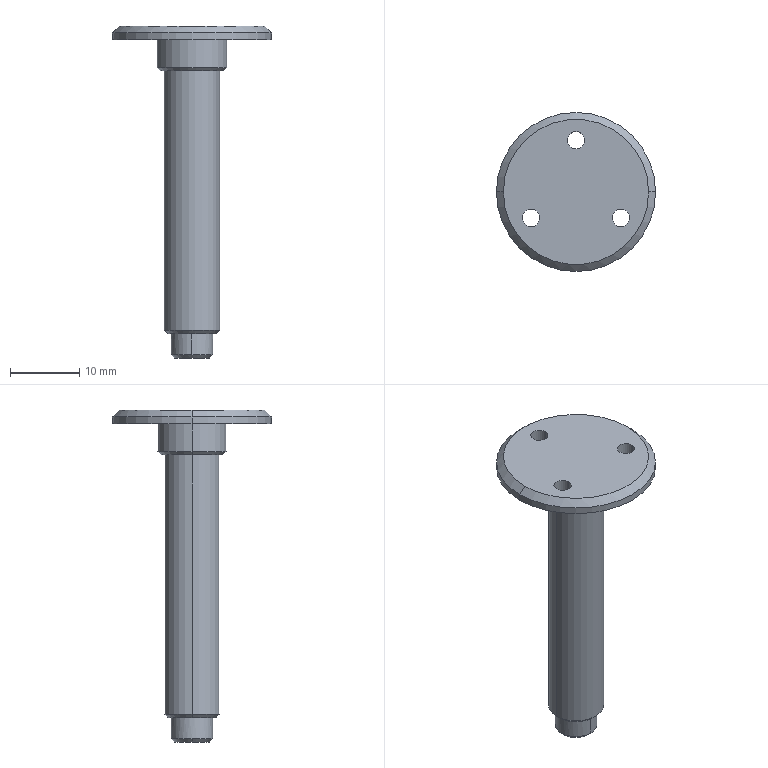Part | NX | features BREP 1 | 1 solid | 30 faces | box 23 x 23 x 48 mm | volume 3023 mm3 | cylinder 16 | cone 8 | plane 6 | commonest cylinder face diameters 2.5 x6 3.2 x2 6 x2 8 x2 10 x2 23 x2
STEP:
#1=CARTESIAN_POINT('',(100.41,208.217,0.));
#2=VERTEX_POINT('',#1);
#3=CARTESIAN_POINT('',(109.41,208.217,0.));
#4=VERTEX_POINT('',#3);
#5=CARTESIAN_POINT('',(104.91,208.217,0.));
#6=DIRECTION('',(0.,0.,-1.));
#7=DIRECTION('',(1.,0.,0.));
#8=AXIS2_PLACEMENT_3D('',#5,#6,#7);
#9=CIRCLE('',#8,4.5);
#10=EDGE_CURVE('',#2,#4,#9,.T.);
#11=ORIENTED_EDGE('',*,*,#10,.F.);
#12=CARTESIAN_POINT('',(99.91,208.217,0.5));
#13=VERTEX_POINT('',#12);
#14=CARTESIAN_POINT('',(99.91,208.217,0.5));
#15=DIRECTION('',(-0.7071,0.,0.7071));
#16=VECTOR('',#15,1000.);
#17=LINE('',#14,#16);
#18=EDGE_CURVE('',#2,#13,#17,.T.);
#19=ORIENTED_EDGE('',*,*,#18,.T.);
#20=CARTESIAN_POINT('',(109.91,208.217,0.5));
#21=VERTEX_POINT('',#20);
#22=CARTESIAN_POINT('',(104.91,208.217,0.5));
#23=DIRECTION('',(0.,0.,1.));
#24=DIRECTION('',(1.,0.,0.));
#25=AXIS2_PLACEMENT_3D('',#22,#23,#24);
#26=CIRCLE('',#25,5.);
#27=EDGE_CURVE('',#21,#13,#26,.T.);
#28=ORIENTED_EDGE('',*,*,#27,.F.);
#29=CARTESIAN_POINT('',(109.91,208.217,0.5));
#30=DIRECTION('',(0.7071,0.,0.7071));
#31=VECTOR('',#30,1000.);
#32=LINE('',#29,#31);
#33=EDGE_CURVE('',#4,#21,#32,.T.);
#34=ORIENTED_EDGE('',*,*,#33,.F.);
#35=EDGE_LOOP('',(#11,#19,#28,#34));
#36=FACE_BOUND('',#35,.T.);
#37=CARTESIAN_POINT('',(104.91,208.217,0.5));
#38=DIRECTION('',(0.,0.,1.));
#39=DIRECTION('',(-1.,0.,0.));
#40=AXIS2_PLACEMENT_3D('',#37,#38,#39);
#41=CONICAL_SURFACE('',#40,5.,0.7854);
#42=ADVANCED_FACE('',(#36),#41,.T.);
#43=CARTESIAN_POINT('',(102.41,208.217,-41.5));
#44=VERTEX_POINT('',#43);
#45=CARTESIAN_POINT('',(107.41,208.217,-41.5));
#46=VERTEX_POINT('',#45);
#47=CARTESIAN_POINT('',(104.91,208.217,-41.5));
#48=DIRECTION('',(0.,0.,-1.));
#49=DIRECTION('',(0.,1.,0.));
#50=AXIS2_PLACEMENT_3D('',#47,#48,#49);
#51=CIRCLE('',#50,2.5);
#52=EDGE_CURVE('',#44,#46,#51,.T.);
#53=ORIENTED_EDGE('',*,*,#52,.F.);
#54=CARTESIAN_POINT('',(101.91,208.217,-41.));
#55=VERTEX_POINT('',#54);
#56=CARTESIAN_POINT('',(102.41,208.217,-41.5));
#57=DIRECTION('',(-0.7071,0.,0.7071));
#58=VECTOR('',#57,1000.);
#59=LINE('',#56,#58);
#60=EDGE_CURVE('',#44,#55,#59,.T.);
#61=ORIENTED_EDGE('',*,*,#60,.T.);
#62=CARTESIAN_POINT('',(104.91,211.217,-41.));
#63=VERTEX_POINT('',#62);
#64=CARTESIAN_POINT('',(104.91,208.217,-41.));
#65=DIRECTION('',(0.,0.,1.));
#66=DIRECTION('',(-1.,0.,0.));
#67=AXIS2_PLACEMENT_3D('',#64,#65,#66);
#68=CIRCLE('',#67,3.);
#69=EDGE_CURVE('',#63,#55,#68,.T.);
#70=ORIENTED_EDGE('',*,*,#69,.F.);
#71=CARTESIAN_POINT('',(107.91,208.217,-41.));
#72=VERTEX_POINT('',#71);
#73=CARTESIAN_POINT('',(104.91,208.217,-41.));
#74=DIRECTION('',(0.,0.,1.));
#75=DIRECTION('',(-1.,0.,0.));
#76=AXIS2_PLACEMENT_3D('',#73,#74,#75);
#77=CIRCLE('',#76,3.);
#78=EDGE_CURVE('',#72,#63,#77,.T.);
#79=ORIENTED_EDGE('',*,*,#78,.F.);
#80=CARTESIAN_POINT('',(107.41,208.217,-41.5));
#81=DIRECTION('',(0.7071,0.,0.7071));
#82=VECTOR('',#81,1000.);
#83=LINE('',#80,#82);
#84=EDGE_CURVE('',#46,#72,#83,.T.);
#85=ORIENTED_EDGE('',*,*,#84,.F.);
#86=EDGE_LOOP('',(#53,#61,#70,#79,#85));
#87=FACE_BOUND('',#86,.T.);
#88=CARTESIAN_POINT('',(104.91,208.217,-41.5));
#89=DIRECTION('',(0.,0.,1.));
#90=DIRECTION('',(-1.,0.,0.));
#91=AXIS2_PLACEMENT_3D('',#88,#89,#90);
#92=CONICAL_SURFACE('',#91,2.5,0.7854);
#93=ADVANCED_FACE('',(#87),#92,.T.);
#94=CARTESIAN_POINT('',(101.41,208.217,-38.));
#95=VERTEX_POINT('',#94);
#96=CARTESIAN_POINT('',(108.41,208.217,-38.));
#97=VERTEX_POINT('',#96);
#98=CARTESIAN_POINT('',(104.91,208.217,-38.));
#99=DIRECTION('',(0.,0.,-1.));
#100=DIRECTION('',(0.,1.,0.));
#101=AXIS2_PLACEMENT_3D('',#98,#99,#100);
#102=CIRCLE('',#101,3.5);
#103=EDGE_CURVE('',#95,#97,#102,.T.);
#104=ORIENTED_EDGE('',*,*,#103,.F.);
#105=CARTESIAN_POINT('',(100.91,208.217,-37.5));
#106=VERTEX_POINT('',#105);
#107=CARTESIAN_POINT('',(101.41,208.217,-38.));
#108=DIRECTION('',(-0.7071,0.,0.7071));
#109=VECTOR('',#108,1000.);
#110=LINE('',#107,#109);
#111=EDGE_CURVE('',#95,#106,#110,.T.);
#112=ORIENTED_EDGE('',*,*,#111,.T.);
#113=CARTESIAN_POINT('',(108.91,208.217,-37.5));
#114=VERTEX_POINT('',#113);
#115=CARTESIAN_POINT('',(104.91,208.217,-37.5));
#116=DIRECTION('',(0.,0.,1.));
#117=DIRECTION('',(-1.,0.,0.));
#118=AXIS2_PLACEMENT_3D('',#115,#116,#117);
#119=CIRCLE('',#118,4.);
#120=EDGE_CURVE('',#114,#106,#119,.T.);
#121=ORIENTED_EDGE('',*,*,#120,.F.);
#122=CARTESIAN_POINT('',(108.41,208.217,-38.));
#123=DIRECTION('',(0.7071,0.,0.7071));
#124=VECTOR('',#123,1000.);
#125=LINE('',#122,#124);
#126=EDGE_CURVE('',#97,#114,#125,.T.);
#127=ORIENTED_EDGE('',*,*,#126,.F.);
#128=EDGE_LOOP('',(#104,#112,#121,#127));
#129=FACE_BOUND('',#128,.T.);
#130=CARTESIAN_POINT('',(104.91,208.217,-38.));
#131=DIRECTION('',(0.,0.,1.));
#132=DIRECTION('',(-1.,0.,0.));
#133=AXIS2_PLACEMENT_3D('',#130,#131,#132);
#134=CONICAL_SURFACE('',#133,3.5,0.7854);
#135=ADVANCED_FACE('',(#129),#134,.T.);
#136=CARTESIAN_POINT('',(104.91,206.617,-29.5));
#137=VERTEX_POINT('',#136);
#138=CARTESIAN_POINT('',(104.91,209.817,-29.5));
#139=VERTEX_POINT('',#138);
#140=CARTESIAN_POINT('',(104.91,208.217,-29.5));
#141=DIRECTION('',(0.,0.,-1.));
#142=DIRECTION('',(0.,1.,0.));
#143=AXIS2_PLACEMENT_3D('',#140,#141,#142);
#144=CIRCLE('',#143,1.6);
#145=EDGE_CURVE('',#137,#139,#144,.T.);
#146=ORIENTED_EDGE('',*,*,#145,.F.);
#147=CARTESIAN_POINT('',(104.91,206.617,-41.5));
#148=VERTEX_POINT('',#147);
#149=CARTESIAN_POINT('',(104.91,206.617,-29.5));
#150=DIRECTION('',(0.,0.,-1.));
#151=VECTOR('',#150,1000.);
#152=LINE('',#149,#151);
#153=EDGE_CURVE('',#137,#148,#152,.T.);
#154=ORIENTED_EDGE('',*,*,#153,.T.);
#155=CARTESIAN_POINT('',(104.91,209.817,-41.5));
#156=VERTEX_POINT('',#155);
#157=CARTESIAN_POINT('',(104.91,208.217,-41.5));
#158=DIRECTION('',(0.,0.,-1.));
#159=DIRECTION('',(0.,1.,0.));
#160=AXIS2_PLACEMENT_3D('',#157,#158,#159);
#161=CIRCLE('',#160,1.6);
#162=EDGE_CURVE('',#148,#156,#161,.T.);
#163=ORIENTED_EDGE('',*,*,#162,.T.);
#164=CARTESIAN_POINT('',(104.91,209.817,-29.5));
#165=DIRECTION('',(0.,0.,-1.));
#166=VECTOR('',#165,1000.);
#167=LINE('',#164,#166);
#168=EDGE_CURVE('',#139,#156,#167,.T.);
#169=ORIENTED_EDGE('',*,*,#168,.F.);
#170=EDGE_LOOP('',(#146,#154,#163,#169));
#171=FACE_BOUND('',#170,.T.);
#172=CARTESIAN_POINT('',(104.91,208.217,-29.5));
#173=DIRECTION('',(0.,0.,-1.));
#174=DIRECTION('',(0.,-1.,0.));
#175=AXIS2_PLACEMENT_3D('',#172,#173,#174);
#176=CYLINDRICAL_SURFACE('',#175,1.6);
#177=ADVANCED_FACE('',(#171),#176,.F.);
#178=CARTESIAN_POINT('',(104.91,211.217,-38.));
#179=VERTEX_POINT('',#178);
#180=CARTESIAN_POINT('',(104.91,205.217,-38.));
#181=VERTEX_POINT('',#180);
#182=CARTESIAN_POINT('',(104.91,208.217,-38.));
#183=DIRECTION('',(0.,0.,-1.));
#184=DIRECTION('',(0.5022,0.8648,0.));
#185=AXIS2_PLACEMENT_3D('',#182,#183,#184);
#186=CIRCLE('',#185,3.);
#187=EDGE_CURVE('',#179,#181,#186,.T.);
#188=ORIENTED_EDGE('',*,*,#187,.T.);
#189=CARTESIAN_POINT('',(104.91,205.217,-41.));
#190=VERTEX_POINT('',#189);
#191=CARTESIAN_POINT('',(104.91,205.217,-22.075));
#192=DIRECTION('',(0.,0.,-1.));
#193=VECTOR('',#192,1000.);
#194=LINE('',#191,#193);
#195=EDGE_CURVE('',#181,#190,#194,.T.);
#196=ORIENTED_EDGE('',*,*,#195,.T.);
#197=CARTESIAN_POINT('',(104.91,208.217,-41.));
#198=DIRECTION('',(0.,0.,1.));
#199=DIRECTION('',(-1.,0.,0.));
#200=AXIS2_PLACEMENT_3D('',#197,#198,#199);
#201=CIRCLE('',#200,3.);
#202=EDGE_CURVE('',#190,#72,#201,.T.);
#203=ORIENTED_EDGE('',*,*,#202,.T.);
#204=ORIENTED_EDGE('',*,*,#78,.T.);
#205=CARTESIAN_POINT('',(104.91,211.217,-22.075));
#206=DIRECTION('',(0.,0.,-1.));
#207=VECTOR('',#206,1000.);
#208=LINE('',#205,#207);
#209=EDGE_CURVE('',#179,#63,#208,.T.);
#210=ORIENTED_EDGE('',*,*,#209,.F.);
#211=EDGE_LOOP('',(#188,#196,#203,#204,#210));
#212=FACE_BOUND('',#211,.T.);
#213=CARTESIAN_POINT('',(104.91,208.217,-22.075));
#214=DIRECTION('',(0.,0.,-1.));
#215=DIRECTION('',(0.,-1.,0.));
#216=AXIS2_PLACEMENT_3D('',#213,#214,#215);
#217=CYLINDRICAL_SURFACE('',#216,3.);
#218=ADVANCED_FACE('',(#212),#217,.T.);
#219=CARTESIAN_POINT('',(115.41,208.217,6.5));
#220=VERTEX_POINT('',#219);
#221=CARTESIAN_POINT('',(94.41,208.217,6.5));
#222=VERTEX_POINT('',#221);
#223=CARTESIAN_POINT('',(104.91,208.217,6.5));
#224=DIRECTION('',(0.,0.,1.));
#225=DIRECTION('',(1.,0.,0.));
#226=AXIS2_PLACEMENT_3D('',#223,#224,#225);
#227=CIRCLE('',#226,10.5);
#228=EDGE_CURVE('',#220,#222,#227,.T.);
#229=ORIENTED_EDGE('',*,*,#228,.F.);
#230=CARTESIAN_POINT('',(116.41,208.217,5.5));
#231=VERTEX_POINT('',#230);
#232=CARTESIAN_POINT('',(115.41,208.217,6.5));
#233=DIRECTION('',(0.7071,0.,-0.7071));
#234=VECTOR('',#233,1000.);
#235=LINE('',#232,#234);
#236=EDGE_CURVE('',#231,#220,#235,.F.);
#237=ORIENTED_EDGE('',*,*,#236,.F.);
#238=CARTESIAN_POINT('',(93.41,208.217,5.5));
#239=VERTEX_POINT('',#238);
#240=CARTESIAN_POINT('',(104.91,208.217,5.5));
#241=DIRECTION('',(0.,0.,-1.));
#242=DIRECTION('',(1.,0.,0.));
#243=AXIS2_PLACEMENT_3D('',#240,#241,#242);
#244=CIRCLE('',#243,11.5);
#245=EDGE_CURVE('',#239,#231,#244,.T.);
#246=ORIENTED_EDGE('',*,*,#245,.F.);
#247=CARTESIAN_POINT('',(94.41,208.217,6.5));
#248=DIRECTION('',(-0.7071,0.,-0.7071));
#249=VECTOR('',#248,1000.);
#250=LINE('',#247,#249);
#251=EDGE_CURVE('',#239,#222,#250,.F.);
#252=ORIENTED_EDGE('',*,*,#251,.T.);
#253=EDGE_LOOP('',(#229,#237,#246,#252));
#254=FACE_BOUND('',#253,.T.);
#255=CARTESIAN_POINT('',(104.91,208.217,6.5));
#256=DIRECTION('',(0.,0.,-1.));
#257=DIRECTION('',(1.,0.,0.));
#258=AXIS2_PLACEMENT_3D('',#255,#256,#257);
#259=CONICAL_SURFACE('',#258,10.5,0.7854);
#260=ADVANCED_FACE('',(#254),#259,.T.);
#261=CARTESIAN_POINT('',(97.165,204.467,6.5));
#262=VERTEX_POINT('',#261);
#263=CARTESIAN_POINT('',(99.665,204.467,6.5));
#264=VERTEX_POINT('',#263);
#265=CARTESIAN_POINT('',(98.415,204.467,6.5));
#266=DIRECTION('',(0.,0.,1.));
#267=DIRECTION('',(1.,0.,0.));
#268=AXIS2_PLACEMENT_3D('',#265,#266,#267);
#269=CIRCLE('',#268,1.25);
#270=EDGE_CURVE('',#262,#264,#269,.T.);
#271=ORIENTED_EDGE('',*,*,#270,.T.);
#272=CARTESIAN_POINT('',(99.665,204.467,4.5));
#273=VERTEX_POINT('',#272);
#274=CARTESIAN_POINT('',(99.665,204.467,6.5));
#275=DIRECTION('',(0.,0.,-1.));
#276=VECTOR('',#275,1000.);
#277=LINE('',#274,#276);
#278=EDGE_CURVE('',#273,#264,#277,.F.);
#279=ORIENTED_EDGE('',*,*,#278,.F.);
#280=CARTESIAN_POINT('',(97.165,204.467,4.5));
#281=VERTEX_POINT('',#280);
#282=CARTESIAN_POINT('',(98.415,204.467,4.5));
#283=DIRECTION('',(0.,0.,1.));
#284=DIRECTION('',(1.,0.,0.));
#285=AXIS2_PLACEMENT_3D('',#282,#283,#284);
#286=CIRCLE('',#285,1.25);
#287=EDGE_CURVE('',#281,#273,#286,.T.);
#288=ORIENTED_EDGE('',*,*,#287,.F.);
#289=CARTESIAN_POINT('',(97.165,204.467,6.5));
#290=DIRECTION('',(0.,0.,-1.));
#291=VECTOR('',#290,1000.);
#292=LINE('',#289,#291);
#293=EDGE_CURVE('',#281,#262,#292,.F.);
#294=ORIENTED_EDGE('',*,*,#293,.T.);
#295=EDGE_LOOP('',(#271,#279,#288,#294));
#296=FACE_BOUND('',#295,.T.);
#297=CARTESIAN_POINT('',(98.415,204.467,6.5));
#298=DIRECTION('',(0.,0.,-1.));
#299=DIRECTION('',(1.,0.,0.));
#300=AXIS2_PLACEMENT_3D('',#297,#298,#299);
#301=CYLINDRICAL_SURFACE('',#300,1.25);
#302=ADVANCED_FACE('',(#296),#301,.F.);
#303=CARTESIAN_POINT('',(110.155,204.467,6.5));
#304=VERTEX_POINT('',#303);
#305=CARTESIAN_POINT('',(112.655,204.467,6.5));
#306=VERTEX_POINT('',#305);
#307=CARTESIAN_POINT('',(111.405,204.467,6.5));
#308=DIRECTION('',(0.,0.,1.));
#309=DIRECTION('',(1.,0.,0.));
#310=AXIS2_PLACEMENT_3D('',#307,#308,#309);
#311=CIRCLE('',#310,1.25);
#312=EDGE_CURVE('',#304,#306,#311,.T.);
#313=ORIENTED_EDGE('',*,*,#312,.T.);
#314=CARTESIAN_POINT('',(112.655,204.467,4.5));
#315=VERTEX_POINT('',#314);
#316=CARTESIAN_POINT('',(112.655,204.467,6.5));
#317=DIRECTION('',(0.,0.,-1.));
#318=VECTOR('',#317,1000.);
#319=LINE('',#316,#318);
#320=EDGE_CURVE('',#315,#306,#319,.F.);
#321=ORIENTED_EDGE('',*,*,#320,.F.);
#322=CARTESIAN_POINT('',(110.155,204.467,4.5));
#323=VERTEX_POINT('',#322);
#324=CARTESIAN_POINT('',(111.405,204.467,4.5));
#325=DIRECTION('',(0.,0.,1.));
#326=DIRECTION('',(1.,0.,0.));
#327=AXIS2_PLACEMENT_3D('',#324,#325,#326);
#328=CIRCLE('',#327,1.25);
#329=EDGE_CURVE('',#323,#315,#328,.T.);
#330=ORIENTED_EDGE('',*,*,#329,.F.);
#331=CARTESIAN_POINT('',(110.155,204.467,6.5));
#332=DIRECTION('',(0.,0.,-1.));
#333=VECTOR('',#332,1000.);
#334=LINE('',#331,#333);
#335=EDGE_CURVE('',#323,#304,#334,.F.);
#336=ORIENTED_EDGE('',*,*,#335,.T.);
#337=EDGE_LOOP('',(#313,#321,#330,#336));
#338=FACE_BOUND('',#337,.T.);
#339=CARTESIAN_POINT('',(111.405,204.467,6.5));
#340=DIRECTION('',(0.,0.,-1.));
#341=DIRECTION('',(1.,0.,0.));
#342=AXIS2_PLACEMENT_3D('',#339,#340,#341);
#343=CYLINDRICAL_SURFACE('',#342,1.25);
#344=ADVANCED_FACE('',(#338),#343,.F.);
#345=CARTESIAN_POINT('',(103.66,215.717,6.5));
#346=VERTEX_POINT('',#345);
#347=CARTESIAN_POINT('',(106.16,215.717,6.5));
#348=VERTEX_POINT('',#347);
#349=CARTESIAN_POINT('',(104.91,215.717,6.5));
#350=DIRECTION('',(0.,0.,1.));
#351=DIRECTION('',(1.,0.,0.));
#352=AXIS2_PLACEMENT_3D('',#349,#350,#351);
#353=CIRCLE('',#352,1.25);
#354=EDGE_CURVE('',#346,#348,#353,.T.);
#355=ORIENTED_EDGE('',*,*,#354,.T.);
#356=CARTESIAN_POINT('',(106.16,215.717,4.5));
#357=VERTEX_POINT('',#356);
#358=CARTESIAN_POINT('',(106.16,215.717,6.5));
#359=DIRECTION('',(0.,0.,-1.));
#360=VECTOR('',#359,1000.);
#361=LINE('',#358,#360);
#362=EDGE_CURVE('',#357,#348,#361,.F.);
#363=ORIENTED_EDGE('',*,*,#362,.F.);
#364=CARTESIAN_POINT('',(103.66,215.717,4.5));
#365=VERTEX_POINT('',#364);
#366=CARTESIAN_POINT('',(104.91,215.717,4.5));
#367=DIRECTION('',(0.,0.,1.));
#368=DIRECTION('',(1.,0.,0.));
#369=AXIS2_PLACEMENT_3D('',#366,#367,#368);
#370=CIRCLE('',#369,1.25);
#371=EDGE_CURVE('',#365,#357,#370,.T.);
#372=ORIENTED_EDGE('',*,*,#371,.F.);
#373=CARTESIAN_POINT('',(103.66,215.717,6.5));
#374=DIRECTION('',(0.,0.,-1.));
#375=VECTOR('',#374,1000.);
#376=LINE('',#373,#375);
#377=EDGE_CURVE('',#365,#346,#376,.F.);
#378=ORIENTED_EDGE('',*,*,#377,.T.);
#379=EDGE_LOOP('',(#355,#363,#372,#378));
#380=FACE_BOUND('',#379,.T.);
#381=CARTESIAN_POINT('',(104.91,215.717,6.5));
#382=DIRECTION('',(0.,0.,-1.));
#383=DIRECTION('',(1.,0.,0.));
#384=AXIS2_PLACEMENT_3D('',#381,#382,#383);
#385=CYLINDRICAL_SURFACE('',#384,1.25);
#386=ADVANCED_FACE('',(#380),#385,.F.);
#387=ORIENTED_EDGE('',*,*,#245,.T.);
#388=CARTESIAN_POINT('',(116.41,208.217,4.5));
#389=VERTEX_POINT('',#388);
#390=CARTESIAN_POINT('',(116.41,208.217,6.5));
#391=DIRECTION('',(0.,0.,-1.));
#392=VECTOR('',#391,1000.);
#393=LINE('',#390,#392);
#394=EDGE_CURVE('',#389,#231,#393,.F.);
#395=ORIENTED_EDGE('',*,*,#394,.F.);
#396=CARTESIAN_POINT('',(93.41,208.217,4.5));
#397=VERTEX_POINT('',#396);
#398=CARTESIAN_POINT('',(104.91,208.217,4.5));
#399=DIRECTION('',(0.,0.,1.));
#400=DIRECTION('',(1.,0.,0.));
#401=AXIS2_PLACEMENT_3D('',#398,#399,#400);
#402=CIRCLE('',#401,11.5);
#403=EDGE_CURVE('',#389,#397,#402,.T.);
#404=ORIENTED_EDGE('',*,*,#403,.T.);
#405=CARTESIAN_POINT('',(93.41,208.217,6.5));
#406=DIRECTION('',(0.,0.,-1.));
#407=VECTOR('',#406,1000.);
#408=LINE('',#405,#407);
#409=EDGE_CURVE('',#397,#239,#408,.F.);
#410=ORIENTED_EDGE('',*,*,#409,.T.);
#411=EDGE_LOOP('',(#387,#395,#404,#410));
#412=FACE_BOUND('',#411,.T.);
#413=CARTESIAN_POINT('',(104.91,208.217,6.5));
#414=DIRECTION('',(0.,0.,-1.));
#415=DIRECTION('',(1.,0.,0.));
#416=AXIS2_PLACEMENT_3D('',#413,#414,#415);
#417=CYLINDRICAL_SURFACE('',#416,11.5);
#418=ADVANCED_FACE('',(#412),#417,.T.);
#419=CARTESIAN_POINT('',(99.91,208.217,4.5));
#420=VERTEX_POINT('',#419);
#421=CARTESIAN_POINT('',(109.91,208.217,4.5));
#422=VERTEX_POINT('',#421);
#423=CARTESIAN_POINT('',(104.91,208.217,4.5));
#424=DIRECTION('',(0.,0.,-1.));
#425=DIRECTION('',(0.,1.,0.));
#426=AXIS2_PLACEMENT_3D('',#423,#424,#425);
#427=CIRCLE('',#426,5.);
#428=EDGE_CURVE('',#420,#422,#427,.T.);
#429=ORIENTED_EDGE('',*,*,#428,.T.);
#430=CARTESIAN_POINT('',(109.91,208.217,18.642));
#431=DIRECTION('',(0.,0.,-1.));
#432=VECTOR('',#431,1000.);
#433=LINE('',#430,#432);
#434=EDGE_CURVE('',#21,#422,#433,.F.);
#435=ORIENTED_EDGE('',*,*,#434,.F.);
#436=ORIENTED_EDGE('',*,*,#27,.T.);
#437=CARTESIAN_POINT('',(99.91,208.217,18.642));
#438=DIRECTION('',(0.,0.,-1.));
#439=VECTOR('',#438,1000.);
#440=LINE('',#437,#439);
#441=EDGE_CURVE('',#13,#420,#440,.F.);
#442=ORIENTED_EDGE('',*,*,#441,.T.);
#443=EDGE_LOOP('',(#429,#435,#436,#442));
#444=FACE_BOUND('',#443,.T.);
#445=CARTESIAN_POINT('',(104.91,208.217,18.642));
#446=DIRECTION('',(0.,0.,-1.));
#447=DIRECTION('',(1.,0.,0.));
#448=AXIS2_PLACEMENT_3D('',#445,#446,#447);
#449=CYLINDRICAL_SURFACE('',#448,5.);
#450=ADVANCED_FACE('',(#444),#449,.T.);
#451=ORIENTED_EDGE('',*,*,#120,.T.);
#452=CARTESIAN_POINT('',(100.91,208.217,0.));
#453=VERTEX_POINT('',#452);
#454=CARTESIAN_POINT('',(100.91,208.217,-52.814));
#455=DIRECTION('',(0.,0.,1.));
#456=VECTOR('',#455,1000.);
#457=LINE('',#454,#456);
#458=EDGE_CURVE('',#106,#453,#457,.T.);
#459=ORIENTED_EDGE('',*,*,#458,.T.);
#460=CARTESIAN_POINT('',(108.91,208.217,0.));
#461=VERTEX_POINT('',#460);
#462=CARTESIAN_POINT('',(104.91,208.217,0.));
#463=DIRECTION('',(0.,0.,-1.));
#464=DIRECTION('',(-1.,0.,0.));
#465=AXIS2_PLACEMENT_3D('',#462,#463,#464);
#466=CIRCLE('',#465,4.);
#467=EDGE_CURVE('',#453,#461,#466,.T.);
#468=ORIENTED_EDGE('',*,*,#467,.T.);
#469=CARTESIAN_POINT('',(108.91,208.217,-52.814));
#470=DIRECTION('',(0.,0.,1.));
#471=VECTOR('',#470,1000.);
#472=LINE('',#469,#471);
#473=EDGE_CURVE('',#114,#461,#472,.T.);
#474=ORIENTED_EDGE('',*,*,#473,.F.);
#475=EDGE_LOOP('',(#451,#459,#468,#474));
#476=FACE_BOUND('',#475,.T.);
#477=CARTESIAN_POINT('',(104.91,208.217,-52.814));
#478=DIRECTION('',(0.,0.,1.));
#479=DIRECTION('',(-1.,0.,0.));
#480=AXIS2_PLACEMENT_3D('',#477,#478,#479);
#481=CYLINDRICAL_SURFACE('',#480,4.);
#482=ADVANCED_FACE('',(#476),#481,.T.);
#483=ORIENTED_EDGE('',*,*,#458,.F.);
#484=CARTESIAN_POINT('',(104.91,208.217,-37.5));
#485=DIRECTION('',(0.,0.,1.));
#486=DIRECTION('',(-1.,0.,0.));
#487=AXIS2_PLACEMENT_3D('',#484,#485,#486);
#488=CIRCLE('',#487,4.);
#489=EDGE_CURVE('',#106,#114,#488,.T.);
#490=ORIENTED_EDGE('',*,*,#489,.T.);
#491=ORIENTED_EDGE('',*,*,#473,.T.);
#492=CARTESIAN_POINT('',(104.91,208.217,0.));
#493=DIRECTION('',(0.,0.,-1.));
#494=DIRECTION('',(-1.,0.,0.));
#495=AXIS2_PLACEMENT_3D('',#492,#493,#494);
#496=CIRCLE('',#495,4.);
#497=EDGE_CURVE('',#461,#453,#496,.T.);
#498=ORIENTED_EDGE('',*,*,#497,.T.);
#499=EDGE_LOOP('',(#483,#490,#491,#498));
#500=FACE_BOUND('',#499,.T.);
#501=CARTESIAN_POINT('',(104.91,208.217,-52.814));
#502=DIRECTION('',(0.,0.,1.));
#503=DIRECTION('',(-1.,0.,0.));
#504=AXIS2_PLACEMENT_3D('',#501,#502,#503);
#505=CYLINDRICAL_SURFACE('',#504,4.);
#506=ADVANCED_FACE('',(#500),#505,.T.);
#507=CARTESIAN_POINT('',(104.91,208.217,0.));
#508=DIRECTION('',(0.,0.,-1.));
#509=DIRECTION('',(1.,0.,0.));
#510=AXIS2_PLACEMENT_3D('',#507,#508,#509);
#511=CIRCLE('',#510,4.5);
#512=EDGE_CURVE('',#4,#2,#511,.T.);
#513=ORIENTED_EDGE('',*,*,#512,.T.);
#514=ORIENTED_EDGE('',*,*,#10,.T.);
#515=EDGE_LOOP('',(#513,#514));
#516=FACE_BOUND('',#515,.T.);
#517=ORIENTED_EDGE('',*,*,#497,.F.);
#518=ORIENTED_EDGE('',*,*,#467,.F.);
#519=EDGE_LOOP('',(#517,#518));
#520=FACE_BOUND('',#519,.T.);
#521=CARTESIAN_POINT('',(104.91,208.217,0.));
#522=DIRECTION('',(0.,0.,1.));
#523=DIRECTION('',(-1.,0.,0.));
#524=AXIS2_PLACEMENT_3D('',#521,#522,#523);
#525=PLANE('',#524);
#526=ADVANCED_FACE('',(#516,#520),#525,.F.);
#527=ORIENTED_EDGE('',*,*,#434,.T.);
#528=CARTESIAN_POINT('',(104.91,208.217,4.5));
#529=DIRECTION('',(0.,0.,-1.));
#530=DIRECTION('',(0.,1.,0.));
#531=AXIS2_PLACEMENT_3D('',#528,#529,#530);
#532=CIRCLE('',#531,5.);
#533=EDGE_CURVE('',#422,#420,#532,.T.);
#534=ORIENTED_EDGE('',*,*,#533,.T.);
#535=ORIENTED_EDGE('',*,*,#441,.F.);
#536=CARTESIAN_POINT('',(104.91,208.217,0.5));
#537=DIRECTION('',(0.,0.,1.));
#538=DIRECTION('',(1.,0.,0.));
#539=AXIS2_PLACEMENT_3D('',#536,#537,#538);
#540=CIRCLE('',#539,5.);
#541=EDGE_CURVE('',#13,#21,#540,.T.);
#542=ORIENTED_EDGE('',*,*,#541,.T.);
#543=EDGE_LOOP('',(#527,#534,#535,#542));
#544=FACE_BOUND('',#543,.T.);
#545=CARTESIAN_POINT('',(104.91,208.217,18.642));
#546=DIRECTION('',(0.,0.,-1.));
#547=DIRECTION('',(1.,0.,0.));
#548=AXIS2_PLACEMENT_3D('',#545,#546,#547);
#549=CYLINDRICAL_SURFACE('',#548,5.);
#550=ADVANCED_FACE('',(#544),#549,.T.);
#551=CARTESIAN_POINT('',(104.91,208.217,6.5));
#552=DIRECTION('',(0.,0.,1.));
#553=DIRECTION('',(1.,0.,0.));
#554=AXIS2_PLACEMENT_3D('',#551,#552,#553);
#555=CIRCLE('',#554,10.5);
#556=EDGE_CURVE('',#222,#220,#555,.T.);
#557=ORIENTED_EDGE('',*,*,#556,.T.);
#558=ORIENTED_EDGE('',*,*,#228,.T.);
#559=EDGE_LOOP('',(#557,#558));
#560=FACE_BOUND('',#559,.T.);
#561=ORIENTED_EDGE('',*,*,#312,.F.);
#562=CARTESIAN_POINT('',(111.405,204.467,6.5));
#563=DIRECTION('',(0.,0.,1.));
#564=DIRECTION('',(1.,0.,0.));
#565=AXIS2_PLACEMENT_3D('',#562,#563,#564);
#566=CIRCLE('',#565,1.25);
#567=EDGE_CURVE('',#306,#304,#566,.T.);
#568=ORIENTED_EDGE('',*,*,#567,.F.);
#569=EDGE_LOOP('',(#561,#568));
#570=FACE_BOUND('',#569,.T.);
#571=ORIENTED_EDGE('',*,*,#354,.F.);
#572=CARTESIAN_POINT('',(104.91,215.717,6.5));
#573=DIRECTION('',(0.,0.,1.));
#574=DIRECTION('',(1.,0.,0.));
#575=AXIS2_PLACEMENT_3D('',#572,#573,#574);
#576=CIRCLE('',#575,1.25);
#577=EDGE_CURVE('',#348,#346,#576,.T.);
#578=ORIENTED_EDGE('',*,*,#577,.F.);
#579=EDGE_LOOP('',(#571,#578));
#580=FACE_BOUND('',#579,.T.);
#581=ORIENTED_EDGE('',*,*,#270,.F.);
#582=CARTESIAN_POINT('',(98.415,204.467,6.5));
#583=DIRECTION('',(0.,0.,1.));
#584=DIRECTION('',(1.,0.,0.));
#585=AXIS2_PLACEMENT_3D('',#582,#583,#584);
#586=CIRCLE('',#585,1.25);
#587=EDGE_CURVE('',#264,#262,#586,.T.);
#588=ORIENTED_EDGE('',*,*,#587,.F.);
#589=EDGE_LOOP('',(#581,#588));
#590=FACE_BOUND('',#589,.T.);
#591=CARTESIAN_POINT('',(104.91,208.217,6.5));
#592=DIRECTION('',(0.,0.,1.));
#593=DIRECTION('',(-1.,0.,0.));
#594=AXIS2_PLACEMENT_3D('',#591,#592,#593);
#595=PLANE('',#594);
#596=ADVANCED_FACE('',(#560,#570,#580,#590),#595,.T.);
#597=CARTESIAN_POINT('',(104.91,208.217,4.5));
#598=DIRECTION('',(0.,0.,1.));
#599=DIRECTION('',(1.,0.,0.));
#600=AXIS2_PLACEMENT_3D('',#597,#598,#599);
#601=CIRCLE('',#600,11.5);
#602=EDGE_CURVE('',#397,#389,#601,.T.);
#603=ORIENTED_EDGE('',*,*,#602,.F.);
#604=ORIENTED_EDGE('',*,*,#403,.F.);
#605=EDGE_LOOP('',(#603,#604));
#606=FACE_BOUND('',#605,.T.);
#607=ORIENTED_EDGE('',*,*,#428,.F.);
#608=ORIENTED_EDGE('',*,*,#533,.F.);
#609=EDGE_LOOP('',(#607,#608));
#610=FACE_BOUND('',#609,.T.);
#611=ORIENTED_EDGE('',*,*,#371,.T.);
#612=CARTESIAN_POINT('',(104.91,215.717,4.5));
#613=DIRECTION('',(0.,0.,1.));
#614=DIRECTION('',(1.,0.,0.));
#615=AXIS2_PLACEMENT_3D('',#612,#613,#614);
#616=CIRCLE('',#615,1.25);
#617=EDGE_CURVE('',#357,#365,#616,.T.);
#618=ORIENTED_EDGE('',*,*,#617,.T.);
#619=EDGE_LOOP('',(#611,#618));
#620=FACE_BOUND('',#619,.T.);
#621=ORIENTED_EDGE('',*,*,#329,.T.);
#622=CARTESIAN_POINT('',(111.405,204.467,4.5));
#623=DIRECTION('',(0.,0.,1.));
#624=DIRECTION('',(1.,0.,0.));
#625=AXIS2_PLACEMENT_3D('',#622,#623,#624);
#626=CIRCLE('',#625,1.25);
#627=EDGE_CURVE('',#315,#323,#626,.T.);
#628=ORIENTED_EDGE('',*,*,#627,.T.);
#629=EDGE_LOOP('',(#621,#628));
#630=FACE_BOUND('',#629,.T.);
#631=ORIENTED_EDGE('',*,*,#287,.T.);
#632=CARTESIAN_POINT('',(98.415,204.467,4.5));
#633=DIRECTION('',(0.,0.,1.));
#634=DIRECTION('',(1.,0.,0.));
#635=AXIS2_PLACEMENT_3D('',#632,#633,#634);
#636=CIRCLE('',#635,1.25);
#637=EDGE_CURVE('',#273,#281,#636,.T.);
#638=ORIENTED_EDGE('',*,*,#637,.T.);
#639=EDGE_LOOP('',(#631,#638));
#640=FACE_BOUND('',#639,.T.);
#641=CARTESIAN_POINT('',(104.91,208.217,4.5));
#642=DIRECTION('',(0.,0.,1.));
#643=DIRECTION('',(-1.,0.,0.));
#644=AXIS2_PLACEMENT_3D('',#641,#642,#643);
#645=PLANE('',#644);
#646=ADVANCED_FACE('',(#606,#610,#620,#630,#640),#645,.F.);
#647=ORIENTED_EDGE('',*,*,#394,.T.);
#648=CARTESIAN_POINT('',(104.91,208.217,5.5));
#649=DIRECTION('',(0.,0.,-1.));
#650=DIRECTION('',(1.,0.,0.));
#651=AXIS2_PLACEMENT_3D('',#648,#649,#650);
#652=CIRCLE('',#651,11.5);
#653=EDGE_CURVE('',#231,#239,#652,.T.);
#654=ORIENTED_EDGE('',*,*,#653,.T.);
#655=ORIENTED_EDGE('',*,*,#409,.F.);
#656=ORIENTED_EDGE('',*,*,#602,.T.);
#657=EDGE_LOOP('',(#647,#654,#655,#656));
#658=FACE_BOUND('',#657,.T.);
#659=CARTESIAN_POINT('',(104.91,208.217,6.5));
#660=DIRECTION('',(0.,0.,-1.));
#661=DIRECTION('',(1.,0.,0.));
#662=AXIS2_PLACEMENT_3D('',#659,#660,#661);
#663=CYLINDRICAL_SURFACE('',#662,11.5);
#664=ADVANCED_FACE('',(#658),#663,.T.);
#665=ORIENTED_EDGE('',*,*,#362,.T.);
#666=ORIENTED_EDGE('',*,*,#577,.T.);
#667=ORIENTED_EDGE('',*,*,#377,.F.);
#668=ORIENTED_EDGE('',*,*,#617,.F.);
#669=EDGE_LOOP('',(#665,#666,#667,#668));
#670=FACE_BOUND('',#669,.T.);
#671=CARTESIAN_POINT('',(104.91,215.717,6.5));
#672=DIRECTION('',(0.,0.,-1.));
#673=DIRECTION('',(1.,0.,0.));
#674=AXIS2_PLACEMENT_3D('',#671,#672,#673);
#675=CYLINDRICAL_SURFACE('',#674,1.25);
#676=ADVANCED_FACE('',(#670),#675,.F.);
#677=ORIENTED_EDGE('',*,*,#320,.T.);
#678=ORIENTED_EDGE('',*,*,#567,.T.);
#679=ORIENTED_EDGE('',*,*,#335,.F.);
#680=ORIENTED_EDGE('',*,*,#627,.F.);
#681=EDGE_LOOP('',(#677,#678,#679,#680));
#682=FACE_BOUND('',#681,.T.);
#683=CARTESIAN_POINT('',(111.405,204.467,6.5));
#684=DIRECTION('',(0.,0.,-1.));
#685=DIRECTION('',(1.,0.,0.));
#686=AXIS2_PLACEMENT_3D('',#683,#684,#685);
#687=CYLINDRICAL_SURFACE('',#686,1.25);
#688=ADVANCED_FACE('',(#682),#687,.F.);
#689=ORIENTED_EDGE('',*,*,#278,.T.);
#690=ORIENTED_EDGE('',*,*,#587,.T.);
#691=ORIENTED_EDGE('',*,*,#293,.F.);
#692=ORIENTED_EDGE('',*,*,#637,.F.);
#693=EDGE_LOOP('',(#689,#690,#691,#692));
#694=FACE_BOUND('',#693,.T.);
#695=CARTESIAN_POINT('',(98.415,204.467,6.5));
#696=DIRECTION('',(0.,0.,-1.));
#697=DIRECTION('',(1.,0.,0.));
#698=AXIS2_PLACEMENT_3D('',#695,#696,#697);
#699=CYLINDRICAL_SURFACE('',#698,1.25);
#700=ADVANCED_FACE('',(#694),#699,.F.);
#701=ORIENTED_EDGE('',*,*,#236,.T.);
#702=ORIENTED_EDGE('',*,*,#556,.F.);
#703=ORIENTED_EDGE('',*,*,#251,.F.);
#704=ORIENTED_EDGE('',*,*,#653,.F.);
#705=EDGE_LOOP('',(#701,#702,#703,#704));
#706=FACE_BOUND('',#705,.T.);
#707=CARTESIAN_POINT('',(104.91,208.217,6.5));
#708=DIRECTION('',(0.,0.,-1.));
#709=DIRECTION('',(1.,0.,0.));
#710=AXIS2_PLACEMENT_3D('',#707,#708,#709);
#711=CONICAL_SURFACE('',#710,10.5,0.7854);
#712=ADVANCED_FACE('',(#706),#711,.T.);
#713=CARTESIAN_POINT('',(104.91,208.217,-38.));
#714=DIRECTION('',(0.,0.,-1.));
#715=DIRECTION('',(0.,1.,0.));
#716=AXIS2_PLACEMENT_3D('',#713,#714,#715);
#717=CIRCLE('',#716,3.5);
#718=EDGE_CURVE('',#97,#95,#717,.T.);
#719=ORIENTED_EDGE('',*,*,#718,.T.);
#720=ORIENTED_EDGE('',*,*,#103,.T.);
#721=EDGE_LOOP('',(#719,#720));
#722=FACE_BOUND('',#721,.T.);
#723=ORIENTED_EDGE('',*,*,#187,.F.);
#724=CARTESIAN_POINT('',(104.91,208.217,-38.));
#725=DIRECTION('',(0.,0.,-1.));
#726=DIRECTION('',(0.5022,0.8648,0.));
#727=AXIS2_PLACEMENT_3D('',#724,#725,#726);
#728=CIRCLE('',#727,3.);
#729=EDGE_CURVE('',#181,#179,#728,.T.);
#730=ORIENTED_EDGE('',*,*,#729,.F.);
#731=EDGE_LOOP('',(#723,#730));
#732=FACE_BOUND('',#731,.T.);
#733=CARTESIAN_POINT('',(107.761,242.997,-38.));
#734=DIRECTION('',(0.,0.,-1.));
#735=DIRECTION('',(1.,0.,0.));
#736=AXIS2_PLACEMENT_3D('',#733,#734,#735);
#737=PLANE('',#736);
#738=ADVANCED_FACE('',(#722,#732),#737,.T.);
#739=ORIENTED_EDGE('',*,*,#195,.F.);
#740=ORIENTED_EDGE('',*,*,#729,.T.);
#741=ORIENTED_EDGE('',*,*,#209,.T.);
#742=ORIENTED_EDGE('',*,*,#69,.T.);
#743=CARTESIAN_POINT('',(104.91,208.217,-41.));
#744=DIRECTION('',(0.,0.,1.));
#745=DIRECTION('',(-1.,0.,0.));
#746=AXIS2_PLACEMENT_3D('',#743,#744,#745);
#747=CIRCLE('',#746,3.);
#748=EDGE_CURVE('',#55,#190,#747,.T.);
#749=ORIENTED_EDGE('',*,*,#748,.T.);
#750=EDGE_LOOP('',(#739,#740,#741,#742,#749));
#751=FACE_BOUND('',#750,.T.);
#752=CARTESIAN_POINT('',(104.91,208.217,-22.075));
#753=DIRECTION('',(0.,0.,-1.));
#754=DIRECTION('',(0.,-1.,0.));
#755=AXIS2_PLACEMENT_3D('',#752,#753,#754);
#756=CYLINDRICAL_SURFACE('',#755,3.);
#757=ADVANCED_FACE('',(#751),#756,.T.);
#758=CARTESIAN_POINT('',(104.91,208.217,-29.5));
#759=DIRECTION('',(0.,0.,-1.));
#760=DIRECTION('',(0.,1.,0.));
#761=AXIS2_PLACEMENT_3D('',#758,#759,#760);
#762=CIRCLE('',#761,1.6);
#763=EDGE_CURVE('',#139,#137,#762,.T.);
#764=ORIENTED_EDGE('',*,*,#763,.T.);
#765=ORIENTED_EDGE('',*,*,#145,.T.);
#766=EDGE_LOOP('',(#764,#765));
#767=FACE_BOUND('',#766,.T.);
#768=CARTESIAN_POINT('',(104.91,208.217,-29.5));
#769=DIRECTION('',(0.,0.,-1.));
#770=DIRECTION('',(1.,0.,0.));
#771=AXIS2_PLACEMENT_3D('',#768,#769,#770);
#772=PLANE('',#771);
#773=ADVANCED_FACE('',(#767),#772,.T.);
#774=ORIENTED_EDGE('',*,*,#153,.F.);
#775=ORIENTED_EDGE('',*,*,#763,.F.);
#776=ORIENTED_EDGE('',*,*,#168,.T.);
#777=CARTESIAN_POINT('',(104.91,208.217,-41.5));
#778=DIRECTION('',(0.,0.,-1.));
#779=DIRECTION('',(0.,1.,0.));
#780=AXIS2_PLACEMENT_3D('',#777,#778,#779);
#781=CIRCLE('',#780,1.6);
#782=EDGE_CURVE('',#156,#148,#781,.T.);
#783=ORIENTED_EDGE('',*,*,#782,.T.);
#784=EDGE_LOOP('',(#774,#775,#776,#783));
#785=FACE_BOUND('',#784,.T.);
#786=CARTESIAN_POINT('',(104.91,208.217,-29.5));
#787=DIRECTION('',(0.,0.,-1.));
#788=DIRECTION('',(0.,-1.,0.));
#789=AXIS2_PLACEMENT_3D('',#786,#787,#788);
#790=CYLINDRICAL_SURFACE('',#789,1.6);
#791=ADVANCED_FACE('',(#785),#790,.F.);
#792=CARTESIAN_POINT('',(104.91,208.217,-41.5));
#793=DIRECTION('',(0.,0.,-1.));
#794=DIRECTION('',(0.,1.,0.));
#795=AXIS2_PLACEMENT_3D('',#792,#793,#794);
#796=CIRCLE('',#795,2.5);
#797=EDGE_CURVE('',#46,#44,#796,.T.);
#798=ORIENTED_EDGE('',*,*,#797,.T.);
#799=ORIENTED_EDGE('',*,*,#52,.T.);
#800=EDGE_LOOP('',(#798,#799));
#801=FACE_BOUND('',#800,.T.);
#802=ORIENTED_EDGE('',*,*,#782,.F.);
#803=ORIENTED_EDGE('',*,*,#162,.F.);
#804=EDGE_LOOP('',(#802,#803));
#805=FACE_BOUND('',#804,.T.);
#806=CARTESIAN_POINT('',(59.321,82.481,-41.5));
#807=DIRECTION('',(0.,0.,-1.));
#808=DIRECTION('',(1.,0.,0.));
#809=AXIS2_PLACEMENT_3D('',#806,#807,#808);
#810=PLANE('',#809);
#811=ADVANCED_FACE('',(#801,#805),#810,.T.);
#812=ORIENTED_EDGE('',*,*,#111,.F.);
#813=ORIENTED_EDGE('',*,*,#718,.F.);
#814=ORIENTED_EDGE('',*,*,#126,.T.);
#815=ORIENTED_EDGE('',*,*,#489,.F.);
#816=EDGE_LOOP('',(#812,#813,#814,#815));
#817=FACE_BOUND('',#816,.T.);
#818=CARTESIAN_POINT('',(104.91,208.217,-38.));
#819=DIRECTION('',(0.,0.,1.));
#820=DIRECTION('',(-1.,0.,0.));
#821=AXIS2_PLACEMENT_3D('',#818,#819,#820);
#822=CONICAL_SURFACE('',#821,3.5,0.7854);
#823=ADVANCED_FACE('',(#817),#822,.T.);
#824=ORIENTED_EDGE('',*,*,#60,.F.);
#825=ORIENTED_EDGE('',*,*,#797,.F.);
#826=ORIENTED_EDGE('',*,*,#84,.T.);
#827=ORIENTED_EDGE('',*,*,#202,.F.);
#828=ORIENTED_EDGE('',*,*,#748,.F.);
#829=EDGE_LOOP('',(#824,#825,#826,#827,#828));
#830=FACE_BOUND('',#829,.T.);
#831=CARTESIAN_POINT('',(104.91,208.217,-41.5));
#832=DIRECTION('',(0.,0.,1.));
#833=DIRECTION('',(-1.,0.,0.));
#834=AXIS2_PLACEMENT_3D('',#831,#832,#833);
#835=CONICAL_SURFACE('',#834,2.5,0.7854);
#836=ADVANCED_FACE('',(#830),#835,.T.);
#837=ORIENTED_EDGE('',*,*,#18,.F.);
#838=ORIENTED_EDGE('',*,*,#512,.F.);
#839=ORIENTED_EDGE('',*,*,#33,.T.);
#840=ORIENTED_EDGE('',*,*,#541,.F.);
#841=EDGE_LOOP('',(#837,#838,#839,#840));
#842=FACE_BOUND('',#841,.T.);
#843=CARTESIAN_POINT('',(104.91,208.217,0.5));
#844=DIRECTION('',(0.,0.,1.));
#845=DIRECTION('',(-1.,0.,0.));
#846=AXIS2_PLACEMENT_3D('',#843,#844,#845);
#847=CONICAL_SURFACE('',#846,5.,0.7854);
#848=ADVANCED_FACE('',(#842),#847,.T.);
#849=CLOSED_SHELL('',(#42,#93,#135,#177,#218,#260,#302,#344,#386,#418,#450,#482,#506,#526,#550,#596,#646,#664,#676,#688,#700,#712,#738,#757,#773,#791,#811,#823,#836,#848));
#850=MANIFOLD_SOLID_BREP('',#849);
#851=(LENGTH_UNIT()NAMED_UNIT(*)SI_UNIT(.MILLI.,.METRE.));
#852=UNCERTAINTY_MEASURE_WITH_UNIT(LENGTH_MEASURE(0.00001),#851,'','');
#853=(NAMED_UNIT(*)PLANE_ANGLE_UNIT()SI_UNIT($,.RADIAN.));
#854=(NAMED_UNIT(*)SI_UNIT($,.STERADIAN.)SOLID_ANGLE_UNIT());
#855=(GEOMETRIC_REPRESENTATION_CONTEXT(3)GLOBAL_UNCERTAINTY_ASSIGNED_CONTEXT((#852))GLOBAL_UNIT_ASSIGNED_CONTEXT((#851,#853,#854))REPRESENTATION_CONTEXT('',''));
#856=ADVANCED_BREP_SHAPE_REPRESENTATION('',(#850),#855);